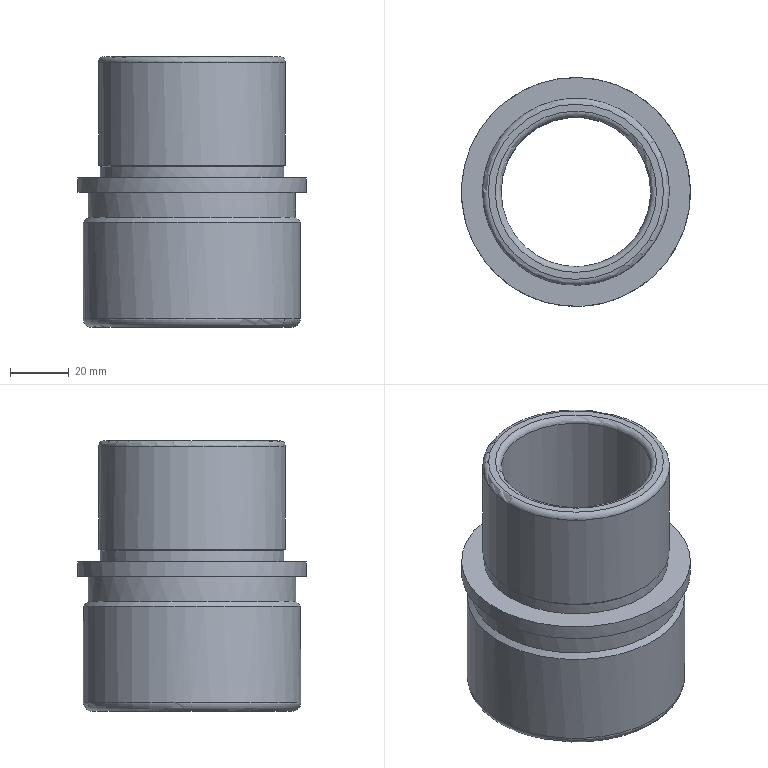Part | STEP file | 1_id1042_x_t | 1 solid | 16 faces | box 77.8 x 77.8 x 92.075 mm | volume 159468 mm3 | cylinder 6 | plane 4 | torus 4 | cone 2 | commonest cylinder face diameters 50.8 x1 62.484 x1 63.5 x1 70.62 x1 73.889 x1 77.8 x1
STEP:
#1=CARTESIAN_POINT('',(0.,0.,0.));
#2=DIRECTION('',(0.,0.,1.));
#3=DIRECTION('',(1.,0.,0.));
#4=AXIS2_PLACEMENT_3D('',#1,#2,#3);
#5=CARTESIAN_POINT('',(983.969,478.443,85.208));
#6=VERTEX_POINT('',#5);
#7=CARTESIAN_POINT('',(908.307,496.557,85.208));
#8=VERTEX_POINT('',#7);
#9=CARTESIAN_POINT('',(946.138,487.5,85.208));
#10=DIRECTION('',(0.,0.,-1.));
#11=DIRECTION('',(0.9725,-0.2328,0.));
#12=AXIS2_PLACEMENT_3D('',#9,#10,#11);
#13=CIRCLE('',#12,38.9);
#14=CARTESIAN_POINT('',(954.359,521.836,85.208));
#15=DIRECTION('',(0.,0.,1.));
#16=DIRECTION('',(0.,1.,0.));
#17=AXIS2_PLACEMENT_3D('',#14,#15,#16);
#18=PLANE('',#17);
#19=CARTESIAN_POINT('',(-43.393,-29.611));
#20=CARTESIAN_POINT('',(-108.918,-13.924));
#21=CARTESIAN_POINT('',(-62.57,34.979));
#22=CARTESIAN_POINT('',(-16.222,83.882));
#23=CARTESIAN_POINT('',(2.955,19.292));
#24=CARTESIAN_POINT('',(22.132,-45.298));
#25=CARTESIAN_POINT('',(-43.393,-29.611));
#26=(BOUNDED_CURVE()B_SPLINE_CURVE(2,(#19,#20,#21,#22,#23,#24,#25),.UNSPECIFIED.,.T.,.F.)B_SPLINE_CURVE_WITH_KNOTS((1,2,2,2,2,1),(-2.094,0.,2.094,4.189,6.283,8.378),.UNSPECIFIED.)CURVE()GEOMETRIC_REPRESENTATION_ITEM()RATIONAL_B_SPLINE_CURVE((1.,0.5,1.,0.5,1.,0.5,1.))REPRESENTATION_ITEM(''));
#27=(GEOMETRIC_REPRESENTATION_CONTEXT(2)PARAMETRIC_REPRESENTATION_CONTEXT()REPRESENTATION_CONTEXT('',''));
#28=DEFINITIONAL_REPRESENTATION('',(#26),#27);
#29=PCURVE('',#18,#28);
#30=CARTESIAN_POINT('',(946.138,487.5,125.11));
#31=DIRECTION('',(0.,0.,-1.));
#32=DIRECTION('',(-0.9725,0.2328,0.));
#33=AXIS2_PLACEMENT_3D('',#30,#31,#32);
#34=CYLINDRICAL_SURFACE('',#33,38.9);
#35=CARTESIAN_POINT('',(3.142,39.902));
#36=DIRECTION('',(1.,0.));
#37=VECTOR('',#36,1.);
#38=LINE('',#35,#37);
#39=(GEOMETRIC_REPRESENTATION_CONTEXT(2)PARAMETRIC_REPRESENTATION_CONTEXT()REPRESENTATION_CONTEXT('',''));
#40=DEFINITIONAL_REPRESENTATION('',(#38),#39);
#41=PCURVE('',#34,#40);
#42=SURFACE_CURVE('',#13,(#29,#41),.PCURVE_S1.);
#43=EDGE_CURVE('',#6,#8,#42,.T.);
#44=ORIENTED_EDGE('',*,*,#43,.T.);
#45=CARTESIAN_POINT('',(946.138,487.5,85.208));
#46=DIRECTION('',(0.,0.,-1.));
#47=DIRECTION('',(0.9725,-0.2328,0.));
#48=AXIS2_PLACEMENT_3D('',#45,#46,#47);
#49=CIRCLE('',#48,38.9);
#50=CARTESIAN_POINT('',(-43.393,-29.611));
#51=CARTESIAN_POINT('',(-108.918,-13.924));
#52=CARTESIAN_POINT('',(-62.57,34.979));
#53=CARTESIAN_POINT('',(-16.222,83.882));
#54=CARTESIAN_POINT('',(2.955,19.292));
#55=CARTESIAN_POINT('',(22.132,-45.298));
#56=CARTESIAN_POINT('',(-43.393,-29.611));
#57=(BOUNDED_CURVE()B_SPLINE_CURVE(2,(#50,#51,#52,#53,#54,#55,#56),.UNSPECIFIED.,.T.,.F.)B_SPLINE_CURVE_WITH_KNOTS((1,2,2,2,2,1),(-2.094,0.,2.094,4.189,6.283,8.378),.UNSPECIFIED.)CURVE()GEOMETRIC_REPRESENTATION_ITEM()RATIONAL_B_SPLINE_CURVE((1.,0.5,1.,0.5,1.,0.5,1.))REPRESENTATION_ITEM(''));
#58=(GEOMETRIC_REPRESENTATION_CONTEXT(2)PARAMETRIC_REPRESENTATION_CONTEXT()REPRESENTATION_CONTEXT('',''));
#59=DEFINITIONAL_REPRESENTATION('',(#57),#58);
#60=PCURVE('',#18,#59);
#61=CARTESIAN_POINT('',(-3.142,39.902));
#62=DIRECTION('',(1.,0.));
#63=VECTOR('',#62,1.);
#64=LINE('',#61,#63);
#65=(GEOMETRIC_REPRESENTATION_CONTEXT(2)PARAMETRIC_REPRESENTATION_CONTEXT()REPRESENTATION_CONTEXT('',''));
#66=DEFINITIONAL_REPRESENTATION('',(#64),#65);
#67=PCURVE('',#34,#66);
#68=SURFACE_CURVE('',#49,(#60,#67),.PCURVE_S1.);
#69=EDGE_CURVE('',#8,#6,#68,.T.);
#70=ORIENTED_EDGE('',*,*,#69,.T.);
#71=EDGE_LOOP('',(#44,#70));
#72=FACE_BOUND('',#71,.T.);
#73=CARTESIAN_POINT('',(980.478,479.279,85.208));
#74=VERTEX_POINT('',#73);
#75=CARTESIAN_POINT('',(946.138,487.5,85.208));
#76=DIRECTION('',(0.,0.,1.));
#77=DIRECTION('',(0.9725,-0.2328,0.));
#78=AXIS2_PLACEMENT_3D('',#75,#76,#77);
#79=CIRCLE('',#78,35.31);
#80=CARTESIAN_POINT('',(-34.336,8.22));
#81=DIRECTION('',(-0.2328,-0.9725));
#82=AXIS2_PLACEMENT_2D('',#80,#81);
#83=CIRCLE('',#82,35.31);
#84=(GEOMETRIC_REPRESENTATION_CONTEXT(2)PARAMETRIC_REPRESENTATION_CONTEXT()REPRESENTATION_CONTEXT('',''));
#85=DEFINITIONAL_REPRESENTATION('',(#83),#84);
#86=PCURVE('',#18,#85);
#87=CARTESIAN_POINT('',(946.138,487.5,76.762));
#88=DIRECTION('',(0.,0.,-1.));
#89=DIRECTION('',(0.9725,-0.2328,0.));
#90=AXIS2_PLACEMENT_3D('',#87,#88,#89);
#91=CYLINDRICAL_SURFACE('',#90,35.31);
#92=CARTESIAN_POINT('',(6.283,-8.446));
#93=DIRECTION('',(-1.,0.));
#94=VECTOR('',#93,1.);
#95=LINE('',#92,#94);
#96=(GEOMETRIC_REPRESENTATION_CONTEXT(2)PARAMETRIC_REPRESENTATION_CONTEXT()REPRESENTATION_CONTEXT('',''));
#97=DEFINITIONAL_REPRESENTATION('',(#95),#96);
#98=PCURVE('',#91,#97);
#99=SURFACE_CURVE('',#79,(#86,#98),.PCURVE_S1.);
#100=EDGE_CURVE('',#74,#74,#99,.T.);
#101=ORIENTED_EDGE('',*,*,#100,.T.);
#102=EDGE_LOOP('',(#101));
#103=FACE_BOUND('',#102,.T.);
#104=ADVANCED_FACE('',(#72,#103),#18,.F.);
#105=ORIENTED_EDGE('',*,*,#69,.F.);
#106=CARTESIAN_POINT('',(908.307,496.557,90.11));
#107=VERTEX_POINT('',#106);
#108=CARTESIAN_POINT('',(908.307,496.557,90.11));
#109=CARTESIAN_POINT('',(908.307,496.557,85.208));
#110=B_SPLINE_CURVE_WITH_KNOTS('',1,(#108,#109),.UNSPECIFIED.,.F.,.F.,(2,2),(35.,39.902),.PIECEWISE_BEZIER_KNOTS.);
#111=CARTESIAN_POINT('',(0.,0.));
#112=DIRECTION('',(0.,1.));
#113=VECTOR('',#112,1.);
#114=LINE('',#111,#113);
#115=(GEOMETRIC_REPRESENTATION_CONTEXT(2)PARAMETRIC_REPRESENTATION_CONTEXT()REPRESENTATION_CONTEXT('',''));
#116=DEFINITIONAL_REPRESENTATION('',(#114),#115);
#117=PCURVE('',#34,#116);
#118=CARTESIAN_POINT('',(6.283,0.));
#119=DIRECTION('',(0.,1.));
#120=VECTOR('',#119,1.);
#121=LINE('',#118,#120);
#122=(GEOMETRIC_REPRESENTATION_CONTEXT(2)PARAMETRIC_REPRESENTATION_CONTEXT()REPRESENTATION_CONTEXT('',''));
#123=DEFINITIONAL_REPRESENTATION('',(#121),#122);
#124=PCURVE('',#34,#123);
#125=SEAM_CURVE('',#110,(#117,#124),.PCURVE_S1.);
#126=EDGE_CURVE('',#107,#8,#125,.T.);
#127=ORIENTED_EDGE('',*,*,#126,.F.);
#128=CARTESIAN_POINT('',(946.138,487.5,90.11));
#129=DIRECTION('',(0.,0.,1.));
#130=DIRECTION('',(-0.9725,0.2328,0.));
#131=AXIS2_PLACEMENT_3D('',#128,#129,#130);
#132=CIRCLE('',#131,38.9);
#133=CARTESIAN_POINT('',(6.283,35.));
#134=DIRECTION('',(-1.,0.));
#135=VECTOR('',#134,1.);
#136=LINE('',#133,#135);
#137=(GEOMETRIC_REPRESENTATION_CONTEXT(2)PARAMETRIC_REPRESENTATION_CONTEXT()REPRESENTATION_CONTEXT('',''));
#138=DEFINITIONAL_REPRESENTATION('',(#136),#137);
#139=PCURVE('',#34,#138);
#140=CARTESIAN_POINT('',(954.869,523.969,90.11));
#141=DIRECTION('',(0.,0.,-1.));
#142=DIRECTION('',(0.,-1.,0.));
#143=AXIS2_PLACEMENT_3D('',#140,#141,#142);
#144=PLANE('',#143);
#145=CARTESIAN_POINT('',(27.413,46.562));
#146=CARTESIAN_POINT('',(92.938,62.249));
#147=CARTESIAN_POINT('',(73.76,-2.341));
#148=CARTESIAN_POINT('',(54.583,-66.931));
#149=CARTESIAN_POINT('',(8.235,-18.028));
#150=CARTESIAN_POINT('',(-38.113,30.875));
#151=CARTESIAN_POINT('',(27.413,46.562));
#152=(BOUNDED_CURVE()B_SPLINE_CURVE(2,(#145,#146,#147,#148,#149,#150,#151),.UNSPECIFIED.,.T.,.F.)B_SPLINE_CURVE_WITH_KNOTS((1,2,2,2,2,1),(-2.094,0.,2.094,4.189,6.283,8.378),.UNSPECIFIED.)CURVE()GEOMETRIC_REPRESENTATION_ITEM()RATIONAL_B_SPLINE_CURVE((1.,0.5,1.,0.5,1.,0.5,1.))REPRESENTATION_ITEM(''));
#153=(GEOMETRIC_REPRESENTATION_CONTEXT(2)PARAMETRIC_REPRESENTATION_CONTEXT()REPRESENTATION_CONTEXT('',''));
#154=DEFINITIONAL_REPRESENTATION('',(#152),#153);
#155=PCURVE('',#144,#154);
#156=SURFACE_CURVE('',#132,(#139,#155),.PCURVE_S1.);
#157=EDGE_CURVE('',#107,#107,#156,.T.);
#158=ORIENTED_EDGE('',*,*,#157,.F.);
#159=ORIENTED_EDGE('',*,*,#126,.T.);
#160=ORIENTED_EDGE('',*,*,#43,.F.);
#161=EDGE_LOOP('',(#105,#127,#158,#159,#160));
#162=FACE_BOUND('',#161,.T.);
#163=ADVANCED_FACE('',(#162),#34,.T.);
#164=ORIENTED_EDGE('',*,*,#157,.T.);
#165=EDGE_LOOP('',(#164));
#166=FACE_BOUND('',#165,.T.);
#167=CARTESIAN_POINT('',(976.522,480.226,90.11));
#168=VERTEX_POINT('',#167);
#169=CARTESIAN_POINT('',(915.755,494.774,90.11));
#170=VERTEX_POINT('',#169);
#171=CARTESIAN_POINT('',(946.138,487.5,90.11));
#172=DIRECTION('',(0.,0.,-1.));
#173=DIRECTION('',(0.9725,-0.2328,0.));
#174=AXIS2_PLACEMENT_3D('',#171,#172,#173);
#175=CIRCLE('',#174,31.242);
#176=CARTESIAN_POINT('',(36.469,8.731));
#177=DIRECTION('',(0.2328,-0.9725));
#178=AXIS2_PLACEMENT_2D('',#176,#177);
#179=CIRCLE('',#178,31.242);
#180=(GEOMETRIC_REPRESENTATION_CONTEXT(2)PARAMETRIC_REPRESENTATION_CONTEXT()REPRESENTATION_CONTEXT('',''));
#181=DEFINITIONAL_REPRESENTATION('',(#179),#180);
#182=PCURVE('',#144,#181);
#183=CARTESIAN_POINT('',(946.138,487.5,125.11));
#184=DIRECTION('',(0.,0.,-1.));
#185=DIRECTION('',(-0.9725,0.2328,0.));
#186=AXIS2_PLACEMENT_3D('',#183,#184,#185);
#187=CYLINDRICAL_SURFACE('',#186,31.242);
#188=CARTESIAN_POINT('',(3.142,35.));
#189=DIRECTION('',(1.,0.));
#190=VECTOR('',#189,1.);
#191=LINE('',#188,#190);
#192=(GEOMETRIC_REPRESENTATION_CONTEXT(2)PARAMETRIC_REPRESENTATION_CONTEXT()REPRESENTATION_CONTEXT('',''));
#193=DEFINITIONAL_REPRESENTATION('',(#191),#192);
#194=PCURVE('',#187,#193);
#195=SURFACE_CURVE('',#175,(#182,#194),.PCURVE_S1.);
#196=EDGE_CURVE('',#168,#170,#195,.T.);
#197=ORIENTED_EDGE('',*,*,#196,.T.);
#198=CARTESIAN_POINT('',(946.138,487.5,90.11));
#199=DIRECTION('',(0.,0.,-1.));
#200=DIRECTION('',(0.9725,-0.2328,0.));
#201=AXIS2_PLACEMENT_3D('',#198,#199,#200);
#202=CIRCLE('',#201,31.242);
#203=CARTESIAN_POINT('',(36.469,8.731));
#204=DIRECTION('',(0.2328,-0.9725));
#205=AXIS2_PLACEMENT_2D('',#203,#204);
#206=CIRCLE('',#205,31.242);
#207=(GEOMETRIC_REPRESENTATION_CONTEXT(2)PARAMETRIC_REPRESENTATION_CONTEXT()REPRESENTATION_CONTEXT('',''));
#208=DEFINITIONAL_REPRESENTATION('',(#206),#207);
#209=PCURVE('',#144,#208);
#210=CARTESIAN_POINT('',(-3.142,35.));
#211=DIRECTION('',(1.,0.));
#212=VECTOR('',#211,1.);
#213=LINE('',#210,#212);
#214=(GEOMETRIC_REPRESENTATION_CONTEXT(2)PARAMETRIC_REPRESENTATION_CONTEXT()REPRESENTATION_CONTEXT('',''));
#215=DEFINITIONAL_REPRESENTATION('',(#213),#214);
#216=PCURVE('',#187,#215);
#217=SURFACE_CURVE('',#202,(#209,#216),.PCURVE_S1.);
#218=EDGE_CURVE('',#170,#168,#217,.T.);
#219=ORIENTED_EDGE('',*,*,#218,.T.);
#220=EDGE_LOOP('',(#197,#219));
#221=FACE_BOUND('',#220,.T.);
#222=ADVANCED_FACE('',(#166,#221),#144,.F.);
#223=ORIENTED_EDGE('',*,*,#218,.F.);
#224=CARTESIAN_POINT('',(915.755,494.774,93.93));
#225=VERTEX_POINT('',#224);
#226=CARTESIAN_POINT('',(915.755,494.774,93.93));
#227=CARTESIAN_POINT('',(915.755,494.774,90.11));
#228=B_SPLINE_CURVE_WITH_KNOTS('',1,(#226,#227),.UNSPECIFIED.,.F.,.F.,(2,2),(31.18,35.),.PIECEWISE_BEZIER_KNOTS.);
#229=CARTESIAN_POINT('',(0.,0.));
#230=DIRECTION('',(0.,1.));
#231=VECTOR('',#230,1.);
#232=LINE('',#229,#231);
#233=(GEOMETRIC_REPRESENTATION_CONTEXT(2)PARAMETRIC_REPRESENTATION_CONTEXT()REPRESENTATION_CONTEXT('',''));
#234=DEFINITIONAL_REPRESENTATION('',(#232),#233);
#235=PCURVE('',#187,#234);
#236=CARTESIAN_POINT('',(6.283,0.));
#237=DIRECTION('',(0.,1.));
#238=VECTOR('',#237,1.);
#239=LINE('',#236,#238);
#240=(GEOMETRIC_REPRESENTATION_CONTEXT(2)PARAMETRIC_REPRESENTATION_CONTEXT()REPRESENTATION_CONTEXT('',''));
#241=DEFINITIONAL_REPRESENTATION('',(#239),#240);
#242=PCURVE('',#187,#241);
#243=SEAM_CURVE('',#228,(#235,#242),.PCURVE_S1.);
#244=EDGE_CURVE('',#225,#170,#243,.T.);
#245=ORIENTED_EDGE('',*,*,#244,.F.);
#246=CARTESIAN_POINT('',(946.138,487.5,93.93));
#247=DIRECTION('',(0.,0.,1.));
#248=DIRECTION('',(-0.9725,0.2328,0.));
#249=AXIS2_PLACEMENT_3D('',#246,#247,#248);
#250=CIRCLE('',#249,31.242);
#251=CARTESIAN_POINT('',(6.283,31.18));
#252=DIRECTION('',(-1.,0.));
#253=VECTOR('',#252,1.);
#254=LINE('',#251,#253);
#255=(GEOMETRIC_REPRESENTATION_CONTEXT(2)PARAMETRIC_REPRESENTATION_CONTEXT()REPRESENTATION_CONTEXT('',''));
#256=DEFINITIONAL_REPRESENTATION('',(#254),#255);
#257=PCURVE('',#187,#256);
#258=CARTESIAN_POINT('',(946.138,487.5,94.184));
#259=DIRECTION('',(0.,0.,1.));
#260=DIRECTION('',(-0.9725,0.2328,0.));
#261=AXIS2_PLACEMENT_3D('',#258,#259,#260);
#262=CONICAL_SURFACE('',#261,31.496,0.7854);
#263=CARTESIAN_POINT('',(0.,-0.254));
#264=DIRECTION('',(1.,0.));
#265=VECTOR('',#264,1.);
#266=LINE('',#263,#265);
#267=(GEOMETRIC_REPRESENTATION_CONTEXT(2)PARAMETRIC_REPRESENTATION_CONTEXT()REPRESENTATION_CONTEXT('',''));
#268=DEFINITIONAL_REPRESENTATION('',(#266),#267);
#269=PCURVE('',#262,#268);
#270=SURFACE_CURVE('',#250,(#257,#269),.PCURVE_S1.);
#271=EDGE_CURVE('',#225,#225,#270,.T.);
#272=ORIENTED_EDGE('',*,*,#271,.F.);
#273=ORIENTED_EDGE('',*,*,#244,.T.);
#274=ORIENTED_EDGE('',*,*,#196,.F.);
#275=EDGE_LOOP('',(#223,#245,#272,#273,#274));
#276=FACE_BOUND('',#275,.T.);
#277=ADVANCED_FACE('',(#276),#187,.T.);
#278=CARTESIAN_POINT('',(915.261,494.892,94.438));
#279=VERTEX_POINT('',#278);
#280=CARTESIAN_POINT('',(946.138,487.5,94.438));
#281=DIRECTION('',(0.,0.,-1.));
#282=DIRECTION('',(-0.9725,0.2328,0.));
#283=AXIS2_PLACEMENT_3D('',#280,#281,#282);
#284=CIRCLE('',#283,31.75);
#285=CARTESIAN_POINT('',(6.283,0.254));
#286=DIRECTION('',(-1.,0.));
#287=VECTOR('',#286,1.);
#288=LINE('',#285,#287);
#289=(GEOMETRIC_REPRESENTATION_CONTEXT(2)PARAMETRIC_REPRESENTATION_CONTEXT()REPRESENTATION_CONTEXT('',''));
#290=DEFINITIONAL_REPRESENTATION('',(#288),#289);
#291=PCURVE('',#262,#290);
#292=CARTESIAN_POINT('',(946.138,487.5,133.047));
#293=DIRECTION('',(0.,0.,-1.));
#294=DIRECTION('',(-0.9725,0.2328,0.));
#295=AXIS2_PLACEMENT_3D('',#292,#293,#294);
#296=CYLINDRICAL_SURFACE('',#295,31.75);
#297=CARTESIAN_POINT('',(0.,38.61));
#298=DIRECTION('',(1.,0.));
#299=VECTOR('',#298,1.);
#300=LINE('',#297,#299);
#301=(GEOMETRIC_REPRESENTATION_CONTEXT(2)PARAMETRIC_REPRESENTATION_CONTEXT()REPRESENTATION_CONTEXT('',''));
#302=DEFINITIONAL_REPRESENTATION('',(#300),#301);
#303=PCURVE('',#296,#302);
#304=SURFACE_CURVE('',#284,(#291,#303),.PCURVE_S1.);
#305=EDGE_CURVE('',#279,#279,#304,.T.);
#306=ORIENTED_EDGE('',*,*,#305,.T.);
#307=CARTESIAN_POINT('',(915.755,494.774,93.93));
#308=CARTESIAN_POINT('',(915.261,494.892,94.438));
#309=B_SPLINE_CURVE_WITH_KNOTS('',1,(#307,#308),.UNSPECIFIED.,.F.,.F.,(2,2),(-0.3592,0.3592),.PIECEWISE_BEZIER_KNOTS.);
#310=CARTESIAN_POINT('',(0.,0.));
#311=DIRECTION('',(0.,1.));
#312=VECTOR('',#311,1.);
#313=LINE('',#310,#312);
#314=(GEOMETRIC_REPRESENTATION_CONTEXT(2)PARAMETRIC_REPRESENTATION_CONTEXT()REPRESENTATION_CONTEXT('',''));
#315=DEFINITIONAL_REPRESENTATION('',(#313),#314);
#316=PCURVE('',#262,#315);
#317=CARTESIAN_POINT('',(6.283,0.));
#318=DIRECTION('',(0.,1.));
#319=VECTOR('',#318,1.);
#320=LINE('',#317,#319);
#321=(GEOMETRIC_REPRESENTATION_CONTEXT(2)PARAMETRIC_REPRESENTATION_CONTEXT()REPRESENTATION_CONTEXT('',''));
#322=DEFINITIONAL_REPRESENTATION('',(#320),#321);
#323=PCURVE('',#262,#322);
#324=SEAM_CURVE('',#309,(#316,#323),.PCURVE_S1.);
#325=EDGE_CURVE('',#225,#279,#324,.T.);
#326=ORIENTED_EDGE('',*,*,#325,.F.);
#327=ORIENTED_EDGE('',*,*,#271,.T.);
#328=ORIENTED_EDGE('',*,*,#325,.T.);
#329=EDGE_LOOP('',(#306,#326,#327,#328));
#330=FACE_BOUND('',#329,.T.);
#331=ADVANCED_FACE('',(#330),#262,.T.);
#332=ORIENTED_EDGE('',*,*,#305,.F.);
#333=CARTESIAN_POINT('',(915.261,494.892,129.385));
#334=VERTEX_POINT('',#333);
#335=CARTESIAN_POINT('',(915.261,494.892,129.385));
#336=CARTESIAN_POINT('',(915.261,494.892,94.438));
#337=B_SPLINE_CURVE_WITH_KNOTS('',1,(#335,#336),.UNSPECIFIED.,.F.,.F.,(2,2),(3.663,38.61),.PIECEWISE_BEZIER_KNOTS.);
#338=CARTESIAN_POINT('',(0.,0.));
#339=DIRECTION('',(0.,1.));
#340=VECTOR('',#339,1.);
#341=LINE('',#338,#340);
#342=(GEOMETRIC_REPRESENTATION_CONTEXT(2)PARAMETRIC_REPRESENTATION_CONTEXT()REPRESENTATION_CONTEXT('',''));
#343=DEFINITIONAL_REPRESENTATION('',(#341),#342);
#344=PCURVE('',#296,#343);
#345=CARTESIAN_POINT('',(6.283,0.));
#346=DIRECTION('',(0.,1.));
#347=VECTOR('',#346,1.);
#348=LINE('',#345,#347);
#349=(GEOMETRIC_REPRESENTATION_CONTEXT(2)PARAMETRIC_REPRESENTATION_CONTEXT()REPRESENTATION_CONTEXT('',''));
#350=DEFINITIONAL_REPRESENTATION('',(#348),#349);
#351=PCURVE('',#296,#350);
#352=SEAM_CURVE('',#337,(#344,#351),.PCURVE_S1.);
#353=EDGE_CURVE('',#334,#279,#352,.T.);
#354=ORIENTED_EDGE('',*,*,#353,.F.);
#355=CARTESIAN_POINT('',(977.888,487.5,129.385));
#356=VERTEX_POINT('',#355);
#357=CARTESIAN_POINT('',(946.138,487.5,129.385));
#358=DIRECTION('',(0.,0.,1.));
#359=DIRECTION('',(1.,0.,0.));
#360=AXIS2_PLACEMENT_3D('',#357,#358,#359);
#361=CIRCLE('',#360,31.75);
#362=CARTESIAN_POINT('',(2.907,3.663));
#363=DIRECTION('',(-1.,0.));
#364=VECTOR('',#363,1.);
#365=LINE('',#362,#364);
#366=(GEOMETRIC_REPRESENTATION_CONTEXT(2)PARAMETRIC_REPRESENTATION_CONTEXT()REPRESENTATION_CONTEXT('',''));
#367=DEFINITIONAL_REPRESENTATION('',(#365),#366);
#368=PCURVE('',#296,#367);
#369=CARTESIAN_POINT('',(946.138,487.5,129.385));
#370=DIRECTION('',(0.,0.,-1.));
#371=DIRECTION('',(1.,0.,0.));
#372=AXIS2_PLACEMENT_3D('',#369,#370,#371);
#373=TOROIDAL_SURFACE('',#372,29.75,2.);
#374=CARTESIAN_POINT('',(6.283,6.283));
#375=DIRECTION('',(-1.,0.));
#376=VECTOR('',#375,1.);
#377=LINE('',#374,#376);
#378=(GEOMETRIC_REPRESENTATION_CONTEXT(2)PARAMETRIC_REPRESENTATION_CONTEXT()REPRESENTATION_CONTEXT('',''));
#379=DEFINITIONAL_REPRESENTATION('',(#377),#378);
#380=PCURVE('',#373,#379);
#381=SURFACE_CURVE('',#361,(#368,#380),.PCURVE_S1.);
#382=EDGE_CURVE('',#356,#334,#381,.T.);
#383=ORIENTED_EDGE('',*,*,#382,.F.);
#384=CARTESIAN_POINT('',(946.138,487.5,129.385));
#385=DIRECTION('',(0.,0.,1.));
#386=DIRECTION('',(1.,0.,0.));
#387=AXIS2_PLACEMENT_3D('',#384,#385,#386);
#388=CIRCLE('',#387,31.75);
#389=CARTESIAN_POINT('',(9.19,3.663));
#390=DIRECTION('',(-1.,0.));
#391=VECTOR('',#390,1.);
#392=LINE('',#389,#391);
#393=(GEOMETRIC_REPRESENTATION_CONTEXT(2)PARAMETRIC_REPRESENTATION_CONTEXT()REPRESENTATION_CONTEXT('',''));
#394=DEFINITIONAL_REPRESENTATION('',(#392),#393);
#395=PCURVE('',#296,#394);
#396=CARTESIAN_POINT('',(6.283,6.283));
#397=DIRECTION('',(-1.,0.));
#398=VECTOR('',#397,1.);
#399=LINE('',#396,#398);
#400=(GEOMETRIC_REPRESENTATION_CONTEXT(2)PARAMETRIC_REPRESENTATION_CONTEXT()REPRESENTATION_CONTEXT('',''));
#401=DEFINITIONAL_REPRESENTATION('',(#399),#400);
#402=PCURVE('',#373,#401);
#403=SURFACE_CURVE('',#388,(#395,#402),.PCURVE_S1.);
#404=EDGE_CURVE('',#334,#356,#403,.T.);
#405=ORIENTED_EDGE('',*,*,#404,.F.);
#406=ORIENTED_EDGE('',*,*,#353,.T.);
#407=EDGE_LOOP('',(#332,#354,#383,#405,#406));
#408=FACE_BOUND('',#407,.T.);
#409=ADVANCED_FACE('',(#408),#296,.T.);
#410=ORIENTED_EDGE('',*,*,#382,.T.);
#411=ORIENTED_EDGE('',*,*,#404,.T.);
#412=CARTESIAN_POINT('',(975.888,487.5,131.385));
#413=VERTEX_POINT('',#412);
#414=CARTESIAN_POINT('',(975.888,487.5,131.385));
#415=CARTESIAN_POINT('',(976.423,487.5,131.385));
#416=CARTESIAN_POINT('',(976.944,487.5,131.215));
#417=CARTESIAN_POINT('',(977.392,487.5,130.889));
#418=CARTESIAN_POINT('',(977.718,487.5,130.44));
#419=CARTESIAN_POINT('',(977.888,487.5,129.92));
#420=CARTESIAN_POINT('',(977.888,487.5,129.385));
#421=(BOUNDED_CURVE()B_SPLINE_CURVE(6,(#414,#415,#416,#417,#418,#419,#420),.UNSPECIFIED.,.F.,.F.)B_SPLINE_CURVE_WITH_KNOTS((7,7),(-1.571,0.),.PIECEWISE_BEZIER_KNOTS.)CURVE()GEOMETRIC_REPRESENTATION_ITEM()RATIONAL_B_SPLINE_CURVE((1.031,1.01,0.9979,0.994,0.9979,1.01,1.031))REPRESENTATION_ITEM(''));
#422=CARTESIAN_POINT('',(0.,6.283));
#423=DIRECTION('',(0.,1.));
#424=VECTOR('',#423,1.);
#425=LINE('',#422,#424);
#426=(GEOMETRIC_REPRESENTATION_CONTEXT(2)PARAMETRIC_REPRESENTATION_CONTEXT()REPRESENTATION_CONTEXT('',''));
#427=DEFINITIONAL_REPRESENTATION('',(#425),#426);
#428=PCURVE('',#373,#427);
#429=CARTESIAN_POINT('',(6.283,6.283));
#430=DIRECTION('',(0.,1.));
#431=VECTOR('',#430,1.);
#432=LINE('',#429,#431);
#433=(GEOMETRIC_REPRESENTATION_CONTEXT(2)PARAMETRIC_REPRESENTATION_CONTEXT()REPRESENTATION_CONTEXT('',''));
#434=DEFINITIONAL_REPRESENTATION('',(#432),#433);
#435=PCURVE('',#373,#434);
#436=SEAM_CURVE('',#421,(#428,#435),.PCURVE_S1.);
#437=EDGE_CURVE('',#413,#356,#436,.T.);
#438=ORIENTED_EDGE('',*,*,#437,.F.);
#439=CARTESIAN_POINT('',(916.388,487.5,131.385));
#440=VERTEX_POINT('',#439);
#441=CARTESIAN_POINT('',(946.138,487.5,131.385));
#442=DIRECTION('',(0.,0.,1.));
#443=DIRECTION('',(-1.,0.,0.));
#444=AXIS2_PLACEMENT_3D('',#441,#442,#443);
#445=CIRCLE('',#444,29.75);
#446=CARTESIAN_POINT('',(3.142,4.712));
#447=DIRECTION('',(-1.,0.));
#448=VECTOR('',#447,1.);
#449=LINE('',#446,#448);
#450=(GEOMETRIC_REPRESENTATION_CONTEXT(2)PARAMETRIC_REPRESENTATION_CONTEXT()REPRESENTATION_CONTEXT('',''));
#451=DEFINITIONAL_REPRESENTATION('',(#449),#450);
#452=PCURVE('',#373,#451);
#453=CARTESIAN_POINT('',(953.24,-102.838,131.385));
#454=DIRECTION('',(0.,0.,-1.));
#455=DIRECTION('',(0.,-1.,0.));
#456=AXIS2_PLACEMENT_3D('',#453,#454,#455);
#457=PLANE('',#456);
#458=CARTESIAN_POINT('',(-590.338,36.851));
#459=CARTESIAN_POINT('',(-538.81,36.851));
#460=CARTESIAN_POINT('',(-564.574,-7.774));
#461=CARTESIAN_POINT('',(-590.338,-52.399));
#462=CARTESIAN_POINT('',(-616.102,-7.774));
#463=CARTESIAN_POINT('',(-641.867,36.851));
#464=CARTESIAN_POINT('',(-590.338,36.851));
#465=(BOUNDED_CURVE()B_SPLINE_CURVE(2,(#458,#459,#460,#461,#462,#463,#464),.UNSPECIFIED.,.T.,.F.)B_SPLINE_CURVE_WITH_KNOTS((1,2,2,2,2,1),(-2.094,0.,2.094,4.189,6.283,8.378),.UNSPECIFIED.)CURVE()GEOMETRIC_REPRESENTATION_ITEM()RATIONAL_B_SPLINE_CURVE((1.,0.5,1.,0.5,1.,0.5,1.))REPRESENTATION_ITEM(''));
#466=(GEOMETRIC_REPRESENTATION_CONTEXT(2)PARAMETRIC_REPRESENTATION_CONTEXT()REPRESENTATION_CONTEXT('',''));
#467=DEFINITIONAL_REPRESENTATION('',(#465),#466);
#468=PCURVE('',#457,#467);
#469=SURFACE_CURVE('',#445,(#452,#468),.PCURVE_S1.);
#470=EDGE_CURVE('',#440,#413,#469,.T.);
#471=ORIENTED_EDGE('',*,*,#470,.F.);
#472=CARTESIAN_POINT('',(946.138,487.5,131.385));
#473=DIRECTION('',(0.,0.,1.));
#474=DIRECTION('',(-1.,0.,0.));
#475=AXIS2_PLACEMENT_3D('',#472,#473,#474);
#476=CIRCLE('',#475,29.75);
#477=CARTESIAN_POINT('',(9.425,4.712));
#478=DIRECTION('',(-1.,0.));
#479=VECTOR('',#478,1.);
#480=LINE('',#477,#479);
#481=(GEOMETRIC_REPRESENTATION_CONTEXT(2)PARAMETRIC_REPRESENTATION_CONTEXT()REPRESENTATION_CONTEXT('',''));
#482=DEFINITIONAL_REPRESENTATION('',(#480),#481);
#483=PCURVE('',#373,#482);
#484=CARTESIAN_POINT('',(-590.338,36.851));
#485=CARTESIAN_POINT('',(-538.81,36.851));
#486=CARTESIAN_POINT('',(-564.574,-7.774));
#487=CARTESIAN_POINT('',(-590.338,-52.399));
#488=CARTESIAN_POINT('',(-616.102,-7.774));
#489=CARTESIAN_POINT('',(-641.867,36.851));
#490=CARTESIAN_POINT('',(-590.338,36.851));
#491=(BOUNDED_CURVE()B_SPLINE_CURVE(2,(#484,#485,#486,#487,#488,#489,#490),.UNSPECIFIED.,.T.,.F.)B_SPLINE_CURVE_WITH_KNOTS((1,2,2,2,2,1),(-2.094,0.,2.094,4.189,6.283,8.378),.UNSPECIFIED.)CURVE()GEOMETRIC_REPRESENTATION_ITEM()RATIONAL_B_SPLINE_CURVE((1.,0.5,1.,0.5,1.,0.5,1.))REPRESENTATION_ITEM(''));
#492=(GEOMETRIC_REPRESENTATION_CONTEXT(2)PARAMETRIC_REPRESENTATION_CONTEXT()REPRESENTATION_CONTEXT('',''));
#493=DEFINITIONAL_REPRESENTATION('',(#491),#492);
#494=PCURVE('',#457,#493);
#495=SURFACE_CURVE('',#476,(#483,#494),.PCURVE_S1.);
#496=EDGE_CURVE('',#413,#440,#495,.T.);
#497=ORIENTED_EDGE('',*,*,#496,.F.);
#498=ORIENTED_EDGE('',*,*,#437,.T.);
#499=EDGE_LOOP('',(#410,#411,#438,#471,#497,#498));
#500=FACE_BOUND('',#499,.T.);
#501=ADVANCED_FACE('',(#500),#373,.T.);
#502=ORIENTED_EDGE('',*,*,#470,.T.);
#503=ORIENTED_EDGE('',*,*,#496,.T.);
#504=EDGE_LOOP('',(#502,#503));
#505=FACE_BOUND('',#504,.T.);
#506=CARTESIAN_POINT('',(918.738,487.5,131.385));
#507=VERTEX_POINT('',#506);
#508=CARTESIAN_POINT('',(973.538,487.5,131.385));
#509=VERTEX_POINT('',#508);
#510=CARTESIAN_POINT('',(946.138,487.5,131.385));
#511=DIRECTION('',(0.,0.,-1.));
#512=DIRECTION('',(-1.,0.,0.));
#513=AXIS2_PLACEMENT_3D('',#510,#511,#512);
#514=CIRCLE('',#513,27.4);
#515=CARTESIAN_POINT('',(-590.338,7.101));
#516=DIRECTION('',(0.,1.));
#517=AXIS2_PLACEMENT_2D('',#515,#516);
#518=CIRCLE('',#517,27.4);
#519=(GEOMETRIC_REPRESENTATION_CONTEXT(2)PARAMETRIC_REPRESENTATION_CONTEXT()REPRESENTATION_CONTEXT('',''));
#520=DEFINITIONAL_REPRESENTATION('',(#518),#519);
#521=PCURVE('',#457,#520);
#522=CARTESIAN_POINT('',(946.138,487.5,129.385));
#523=DIRECTION('',(0.,0.,-1.));
#524=DIRECTION('',(1.,0.,0.));
#525=AXIS2_PLACEMENT_3D('',#522,#523,#524);
#526=TOROIDAL_SURFACE('',#525,27.4,2.);
#527=CARTESIAN_POINT('',(3.142,4.712));
#528=DIRECTION('',(1.,0.));
#529=VECTOR('',#528,1.);
#530=LINE('',#527,#529);
#531=(GEOMETRIC_REPRESENTATION_CONTEXT(2)PARAMETRIC_REPRESENTATION_CONTEXT()REPRESENTATION_CONTEXT('',''));
#532=DEFINITIONAL_REPRESENTATION('',(#530),#531);
#533=PCURVE('',#526,#532);
#534=SURFACE_CURVE('',#514,(#521,#533),.PCURVE_S1.);
#535=EDGE_CURVE('',#507,#509,#534,.T.);
#536=ORIENTED_EDGE('',*,*,#535,.T.);
#537=CARTESIAN_POINT('',(946.138,487.5,131.385));
#538=DIRECTION('',(0.,0.,-1.));
#539=DIRECTION('',(-1.,0.,0.));
#540=AXIS2_PLACEMENT_3D('',#537,#538,#539);
#541=CIRCLE('',#540,27.4);
#542=CARTESIAN_POINT('',(-590.338,7.101));
#543=DIRECTION('',(0.,1.));
#544=AXIS2_PLACEMENT_2D('',#542,#543);
#545=CIRCLE('',#544,27.4);
#546=(GEOMETRIC_REPRESENTATION_CONTEXT(2)PARAMETRIC_REPRESENTATION_CONTEXT()REPRESENTATION_CONTEXT('',''));
#547=DEFINITIONAL_REPRESENTATION('',(#545),#546);
#548=PCURVE('',#457,#547);
#549=CARTESIAN_POINT('',(-3.142,4.712));
#550=DIRECTION('',(1.,0.));
#551=VECTOR('',#550,1.);
#552=LINE('',#549,#551);
#553=(GEOMETRIC_REPRESENTATION_CONTEXT(2)PARAMETRIC_REPRESENTATION_CONTEXT()REPRESENTATION_CONTEXT('',''));
#554=DEFINITIONAL_REPRESENTATION('',(#552),#553);
#555=PCURVE('',#526,#554);
#556=SURFACE_CURVE('',#541,(#548,#555),.PCURVE_S1.);
#557=EDGE_CURVE('',#509,#507,#556,.T.);
#558=ORIENTED_EDGE('',*,*,#557,.T.);
#559=EDGE_LOOP('',(#536,#558));
#560=FACE_BOUND('',#559,.T.);
#561=ADVANCED_FACE('',(#505,#560),#457,.F.);
#562=ORIENTED_EDGE('',*,*,#557,.F.);
#563=CARTESIAN_POINT('',(971.538,487.5,129.385));
#564=VERTEX_POINT('',#563);
#565=CARTESIAN_POINT('',(971.538,487.5,129.385));
#566=CARTESIAN_POINT('',(971.538,487.5,129.92));
#567=CARTESIAN_POINT('',(971.708,487.5,130.44));
#568=CARTESIAN_POINT('',(972.035,487.5,130.889));
#569=CARTESIAN_POINT('',(972.483,487.5,131.215));
#570=CARTESIAN_POINT('',(973.004,487.5,131.385));
#571=CARTESIAN_POINT('',(973.538,487.5,131.385));
#572=(BOUNDED_CURVE()B_SPLINE_CURVE(6,(#565,#566,#567,#568,#569,#570,#571),.UNSPECIFIED.,.F.,.F.)B_SPLINE_CURVE_WITH_KNOTS((7,7),(3.142,4.712),.PIECEWISE_BEZIER_KNOTS.)CURVE()GEOMETRIC_REPRESENTATION_ITEM()RATIONAL_B_SPLINE_CURVE((1.031,1.01,0.9979,0.994,0.9979,1.01,1.031))REPRESENTATION_ITEM(''));
#573=CARTESIAN_POINT('',(0.,0.));
#574=DIRECTION('',(0.,1.));
#575=VECTOR('',#574,1.);
#576=LINE('',#573,#575);
#577=(GEOMETRIC_REPRESENTATION_CONTEXT(2)PARAMETRIC_REPRESENTATION_CONTEXT()REPRESENTATION_CONTEXT('',''));
#578=DEFINITIONAL_REPRESENTATION('',(#576),#577);
#579=PCURVE('',#526,#578);
#580=CARTESIAN_POINT('',(6.283,0.));
#581=DIRECTION('',(0.,1.));
#582=VECTOR('',#581,1.);
#583=LINE('',#580,#582);
#584=(GEOMETRIC_REPRESENTATION_CONTEXT(2)PARAMETRIC_REPRESENTATION_CONTEXT()REPRESENTATION_CONTEXT('',''));
#585=DEFINITIONAL_REPRESENTATION('',(#583),#584);
#586=PCURVE('',#526,#585);
#587=SEAM_CURVE('',#572,(#579,#586),.PCURVE_S1.);
#588=EDGE_CURVE('',#564,#509,#587,.T.);
#589=ORIENTED_EDGE('',*,*,#588,.F.);
#590=CARTESIAN_POINT('',(970.84,481.586,129.385));
#591=VERTEX_POINT('',#590);
#592=CARTESIAN_POINT('',(946.138,487.5,129.385));
#593=DIRECTION('',(0.,0.,-1.));
#594=DIRECTION('',(1.,0.,0.));
#595=AXIS2_PLACEMENT_3D('',#592,#593,#594);
#596=CIRCLE('',#595,25.4);
#597=CARTESIAN_POINT('',(0.,3.142));
#598=DIRECTION('',(1.,0.));
#599=VECTOR('',#598,1.);
#600=LINE('',#597,#599);
#601=(GEOMETRIC_REPRESENTATION_CONTEXT(2)PARAMETRIC_REPRESENTATION_CONTEXT()REPRESENTATION_CONTEXT('',''));
#602=DEFINITIONAL_REPRESENTATION('',(#600),#601);
#603=PCURVE('',#526,#602);
#604=CARTESIAN_POINT('',(946.138,487.5,158.047));
#605=DIRECTION('',(0.,0.,1.));
#606=DIRECTION('',(0.9725,-0.2328,0.));
#607=AXIS2_PLACEMENT_3D('',#604,#605,#606);
#608=CYLINDRICAL_SURFACE('',#607,25.4);
#609=CARTESIAN_POINT('',(0.235,-28.663));
#610=DIRECTION('',(-1.,0.));
#611=VECTOR('',#610,1.);
#612=LINE('',#609,#611);
#613=(GEOMETRIC_REPRESENTATION_CONTEXT(2)PARAMETRIC_REPRESENTATION_CONTEXT()REPRESENTATION_CONTEXT('',''));
#614=DEFINITIONAL_REPRESENTATION('',(#612),#613);
#615=PCURVE('',#608,#614);
#616=SURFACE_CURVE('',#596,(#603,#615),.PCURVE_S1.);
#617=EDGE_CURVE('',#564,#591,#616,.T.);
#618=ORIENTED_EDGE('',*,*,#617,.T.);
#619=CARTESIAN_POINT('',(946.138,487.5,129.385));
#620=DIRECTION('',(0.,0.,-1.));
#621=DIRECTION('',(1.,0.,0.));
#622=AXIS2_PLACEMENT_3D('',#619,#620,#621);
#623=CIRCLE('',#622,25.4);
#624=CARTESIAN_POINT('',(0.,3.142));
#625=DIRECTION('',(1.,0.));
#626=VECTOR('',#625,1.);
#627=LINE('',#624,#626);
#628=(GEOMETRIC_REPRESENTATION_CONTEXT(2)PARAMETRIC_REPRESENTATION_CONTEXT()REPRESENTATION_CONTEXT('',''));
#629=DEFINITIONAL_REPRESENTATION('',(#627),#628);
#630=PCURVE('',#526,#629);
#631=CARTESIAN_POINT('',(6.518,-28.663));
#632=DIRECTION('',(-1.,0.));
#633=VECTOR('',#632,1.);
#634=LINE('',#631,#633);
#635=(GEOMETRIC_REPRESENTATION_CONTEXT(2)PARAMETRIC_REPRESENTATION_CONTEXT()REPRESENTATION_CONTEXT('',''));
#636=DEFINITIONAL_REPRESENTATION('',(#634),#635);
#637=PCURVE('',#608,#636);
#638=SURFACE_CURVE('',#623,(#630,#637),.PCURVE_S1.);
#639=EDGE_CURVE('',#591,#564,#638,.T.);
#640=ORIENTED_EDGE('',*,*,#639,.T.);
#641=ORIENTED_EDGE('',*,*,#588,.T.);
#642=ORIENTED_EDGE('',*,*,#535,.F.);
#643=EDGE_LOOP('',(#562,#589,#618,#640,#641,#642));
#644=FACE_BOUND('',#643,.T.);
#645=ADVANCED_FACE('',(#644),#526,.T.);
#646=ORIENTED_EDGE('',*,*,#617,.T.);
#647=CARTESIAN_POINT('',(970.84,481.586,41.31));
#648=VERTEX_POINT('',#647);
#649=CARTESIAN_POINT('',(970.84,481.586,41.31));
#650=CARTESIAN_POINT('',(970.84,481.586,129.385));
#651=B_SPLINE_CURVE_WITH_KNOTS('',1,(#649,#650),.UNSPECIFIED.,.F.,.F.,(2,2),(-116.738,-28.663),.PIECEWISE_BEZIER_KNOTS.);
#652=CARTESIAN_POINT('',(0.,0.));
#653=DIRECTION('',(0.,1.));
#654=VECTOR('',#653,1.);
#655=LINE('',#652,#654);
#656=(GEOMETRIC_REPRESENTATION_CONTEXT(2)PARAMETRIC_REPRESENTATION_CONTEXT()REPRESENTATION_CONTEXT('',''));
#657=DEFINITIONAL_REPRESENTATION('',(#655),#656);
#658=PCURVE('',#608,#657);
#659=CARTESIAN_POINT('',(6.283,0.));
#660=DIRECTION('',(0.,1.));
#661=VECTOR('',#660,1.);
#662=LINE('',#659,#661);
#663=(GEOMETRIC_REPRESENTATION_CONTEXT(2)PARAMETRIC_REPRESENTATION_CONTEXT()REPRESENTATION_CONTEXT('',''));
#664=DEFINITIONAL_REPRESENTATION('',(#662),#663);
#665=PCURVE('',#608,#664);
#666=SEAM_CURVE('',#651,(#658,#665),.PCURVE_S1.);
#667=EDGE_CURVE('',#648,#591,#666,.T.);
#668=ORIENTED_EDGE('',*,*,#667,.F.);
#669=CARTESIAN_POINT('',(920.738,487.5,41.31));
#670=VERTEX_POINT('',#669);
#671=CARTESIAN_POINT('',(946.138,487.5,41.31));
#672=DIRECTION('',(0.,0.,1.));
#673=DIRECTION('',(0.9725,-0.2328,0.));
#674=AXIS2_PLACEMENT_3D('',#671,#672,#673);
#675=CIRCLE('',#674,25.4);
#676=CARTESIAN_POINT('',(0.,-116.738));
#677=DIRECTION('',(1.,0.));
#678=VECTOR('',#677,1.);
#679=LINE('',#676,#678);
#680=(GEOMETRIC_REPRESENTATION_CONTEXT(2)PARAMETRIC_REPRESENTATION_CONTEXT()REPRESENTATION_CONTEXT('',''));
#681=DEFINITIONAL_REPRESENTATION('',(#679),#680);
#682=PCURVE('',#608,#681);
#683=CARTESIAN_POINT('',(946.138,487.5,41.31));
#684=DIRECTION('',(0.,0.,1.));
#685=DIRECTION('',(-1.,0.,0.));
#686=AXIS2_PLACEMENT_3D('',#683,#684,#685);
#687=TOROIDAL_SURFACE('',#686,27.4,2.);
#688=CARTESIAN_POINT('',(2.907,3.142));
#689=DIRECTION('',(1.,0.));
#690=VECTOR('',#689,1.);
#691=LINE('',#688,#690);
#692=(GEOMETRIC_REPRESENTATION_CONTEXT(2)PARAMETRIC_REPRESENTATION_CONTEXT()REPRESENTATION_CONTEXT('',''));
#693=DEFINITIONAL_REPRESENTATION('',(#691),#692);
#694=PCURVE('',#687,#693);
#695=SURFACE_CURVE('',#675,(#682,#694),.PCURVE_S1.);
#696=EDGE_CURVE('',#648,#670,#695,.T.);
#697=ORIENTED_EDGE('',*,*,#696,.T.);
#698=CARTESIAN_POINT('',(946.138,487.5,41.31));
#699=DIRECTION('',(0.,0.,1.));
#700=DIRECTION('',(0.9725,-0.2328,0.));
#701=AXIS2_PLACEMENT_3D('',#698,#699,#700);
#702=CIRCLE('',#701,25.4);
#703=CARTESIAN_POINT('',(0.,-116.738));
#704=DIRECTION('',(1.,0.));
#705=VECTOR('',#704,1.);
#706=LINE('',#703,#705);
#707=(GEOMETRIC_REPRESENTATION_CONTEXT(2)PARAMETRIC_REPRESENTATION_CONTEXT()REPRESENTATION_CONTEXT('',''));
#708=DEFINITIONAL_REPRESENTATION('',(#706),#707);
#709=PCURVE('',#608,#708);
#710=CARTESIAN_POINT('',(-3.377,3.142));
#711=DIRECTION('',(1.,0.));
#712=VECTOR('',#711,1.);
#713=LINE('',#710,#712);
#714=(GEOMETRIC_REPRESENTATION_CONTEXT(2)PARAMETRIC_REPRESENTATION_CONTEXT()REPRESENTATION_CONTEXT('',''));
#715=DEFINITIONAL_REPRESENTATION('',(#713),#714);
#716=PCURVE('',#687,#715);
#717=SURFACE_CURVE('',#702,(#709,#716),.PCURVE_S1.);
#718=EDGE_CURVE('',#670,#648,#717,.T.);
#719=ORIENTED_EDGE('',*,*,#718,.T.);
#720=ORIENTED_EDGE('',*,*,#667,.T.);
#721=ORIENTED_EDGE('',*,*,#639,.T.);
#722=EDGE_LOOP('',(#646,#668,#697,#719,#720,#721));
#723=FACE_BOUND('',#722,.F.);
#724=ADVANCED_FACE('',(#723),#608,.F.);
#725=CARTESIAN_POINT('',(918.738,487.5,39.31));
#726=VERTEX_POINT('',#725);
#727=CARTESIAN_POINT('',(946.138,487.5,39.31));
#728=DIRECTION('',(0.,0.,1.));
#729=DIRECTION('',(-1.,0.,0.));
#730=AXIS2_PLACEMENT_3D('',#727,#728,#729);
#731=CIRCLE('',#730,27.4);
#732=CARTESIAN_POINT('',(0.,4.712));
#733=DIRECTION('',(1.,0.));
#734=VECTOR('',#733,1.);
#735=LINE('',#732,#734);
#736=(GEOMETRIC_REPRESENTATION_CONTEXT(2)PARAMETRIC_REPRESENTATION_CONTEXT()REPRESENTATION_CONTEXT('',''));
#737=DEFINITIONAL_REPRESENTATION('',(#735),#736);
#738=PCURVE('',#687,#737);
#739=CARTESIAN_POINT('',(946.138,-132.5,39.31));
#740=DIRECTION('',(0.,0.,1.));
#741=DIRECTION('',(0.,1.,0.));
#742=AXIS2_PLACEMENT_3D('',#739,#740,#741);
#743=PLANE('',#742);
#744=CARTESIAN_POINT('',(620.,0.));
#745=DIRECTION('',(0.,1.));
#746=AXIS2_PLACEMENT_2D('',#744,#745);
#747=CIRCLE('',#746,27.4);
#748=(GEOMETRIC_REPRESENTATION_CONTEXT(2)PARAMETRIC_REPRESENTATION_CONTEXT()REPRESENTATION_CONTEXT('',''));
#749=DEFINITIONAL_REPRESENTATION('',(#747),#748);
#750=PCURVE('',#743,#749);
#751=SURFACE_CURVE('',#731,(#738,#750),.PCURVE_S1.);
#752=EDGE_CURVE('',#726,#726,#751,.T.);
#753=ORIENTED_EDGE('',*,*,#752,.F.);
#754=CARTESIAN_POINT('',(920.738,487.5,41.31));
#755=CARTESIAN_POINT('',(920.738,487.5,40.775));
#756=CARTESIAN_POINT('',(920.568,487.5,40.255));
#757=CARTESIAN_POINT('',(920.242,487.5,39.806));
#758=CARTESIAN_POINT('',(919.794,487.5,39.48));
#759=CARTESIAN_POINT('',(919.273,487.5,39.31));
#760=CARTESIAN_POINT('',(918.738,487.5,39.31));
#761=(BOUNDED_CURVE()B_SPLINE_CURVE(6,(#754,#755,#756,#757,#758,#759,#760),.UNSPECIFIED.,.F.,.F.)B_SPLINE_CURVE_WITH_KNOTS((7,7),(3.142,4.712),.PIECEWISE_BEZIER_KNOTS.)CURVE()GEOMETRIC_REPRESENTATION_ITEM()RATIONAL_B_SPLINE_CURVE((1.031,1.01,0.9979,0.994,0.9979,1.01,1.031))REPRESENTATION_ITEM(''));
#762=CARTESIAN_POINT('',(0.,0.));
#763=DIRECTION('',(0.,1.));
#764=VECTOR('',#763,1.);
#765=LINE('',#762,#764);
#766=(GEOMETRIC_REPRESENTATION_CONTEXT(2)PARAMETRIC_REPRESENTATION_CONTEXT()REPRESENTATION_CONTEXT('',''));
#767=DEFINITIONAL_REPRESENTATION('',(#765),#766);
#768=PCURVE('',#687,#767);
#769=CARTESIAN_POINT('',(6.283,0.));
#770=DIRECTION('',(0.,1.));
#771=VECTOR('',#770,1.);
#772=LINE('',#769,#771);
#773=(GEOMETRIC_REPRESENTATION_CONTEXT(2)PARAMETRIC_REPRESENTATION_CONTEXT()REPRESENTATION_CONTEXT('',''));
#774=DEFINITIONAL_REPRESENTATION('',(#772),#773);
#775=PCURVE('',#687,#774);
#776=SEAM_CURVE('',#761,(#768,#775),.PCURVE_S1.);
#777=EDGE_CURVE('',#670,#726,#776,.T.);
#778=ORIENTED_EDGE('',*,*,#777,.F.);
#779=ORIENTED_EDGE('',*,*,#718,.T.);
#780=ORIENTED_EDGE('',*,*,#696,.T.);
#781=ORIENTED_EDGE('',*,*,#777,.T.);
#782=EDGE_LOOP('',(#753,#778,#779,#780,#781));
#783=FACE_BOUND('',#782,.T.);
#784=ADVANCED_FACE('',(#783),#687,.T.);
#785=CARTESIAN_POINT('',(980.083,487.5,39.31));
#786=VERTEX_POINT('',#785);
#787=CARTESIAN_POINT('',(912.194,487.5,39.31));
#788=VERTEX_POINT('',#787);
#789=CARTESIAN_POINT('',(946.138,487.5,39.31));
#790=DIRECTION('',(0.,0.,-1.));
#791=DIRECTION('',(1.,0.,0.));
#792=AXIS2_PLACEMENT_3D('',#789,#790,#791);
#793=CIRCLE('',#792,33.944);
#794=CARTESIAN_POINT('',(620.,-33.944));
#795=CARTESIAN_POINT('',(561.207,-33.944));
#796=CARTESIAN_POINT('',(590.603,16.972));
#797=CARTESIAN_POINT('',(620.,67.889));
#798=CARTESIAN_POINT('',(649.397,16.972));
#799=CARTESIAN_POINT('',(678.793,-33.944));
#800=CARTESIAN_POINT('',(620.,-33.944));
#801=(BOUNDED_CURVE()B_SPLINE_CURVE(2,(#794,#795,#796,#797,#798,#799,#800),.UNSPECIFIED.,.T.,.F.)B_SPLINE_CURVE_WITH_KNOTS((1,2,2,2,2,1),(-2.094,0.,2.094,4.189,6.283,8.378),.UNSPECIFIED.)CURVE()GEOMETRIC_REPRESENTATION_ITEM()RATIONAL_B_SPLINE_CURVE((1.,0.5,1.,0.5,1.,0.5,1.))REPRESENTATION_ITEM(''));
#802=(GEOMETRIC_REPRESENTATION_CONTEXT(2)PARAMETRIC_REPRESENTATION_CONTEXT()REPRESENTATION_CONTEXT('',''));
#803=DEFINITIONAL_REPRESENTATION('',(#801),#802);
#804=PCURVE('',#743,#803);
#805=CARTESIAN_POINT('',(946.138,487.5,42.31));
#806=DIRECTION('',(0.,0.,1.));
#807=DIRECTION('',(-1.,0.,0.));
#808=AXIS2_PLACEMENT_3D('',#805,#806,#807);
#809=TOROIDAL_SURFACE('',#808,33.944,3.);
#810=CARTESIAN_POINT('',(3.142,4.712));
#811=DIRECTION('',(-1.,0.));
#812=VECTOR('',#811,1.);
#813=LINE('',#810,#812);
#814=(GEOMETRIC_REPRESENTATION_CONTEXT(2)PARAMETRIC_REPRESENTATION_CONTEXT()REPRESENTATION_CONTEXT('',''));
#815=DEFINITIONAL_REPRESENTATION('',(#813),#814);
#816=PCURVE('',#809,#815);
#817=SURFACE_CURVE('',#793,(#804,#816),.PCURVE_S1.);
#818=EDGE_CURVE('',#786,#788,#817,.T.);
#819=ORIENTED_EDGE('',*,*,#818,.T.);
#820=CARTESIAN_POINT('',(946.138,487.5,39.31));
#821=DIRECTION('',(0.,0.,-1.));
#822=DIRECTION('',(1.,0.,0.));
#823=AXIS2_PLACEMENT_3D('',#820,#821,#822);
#824=CIRCLE('',#823,33.944);
#825=CARTESIAN_POINT('',(620.,-33.944));
#826=CARTESIAN_POINT('',(561.207,-33.944));
#827=CARTESIAN_POINT('',(590.603,16.972));
#828=CARTESIAN_POINT('',(620.,67.889));
#829=CARTESIAN_POINT('',(649.397,16.972));
#830=CARTESIAN_POINT('',(678.793,-33.944));
#831=CARTESIAN_POINT('',(620.,-33.944));
#832=(BOUNDED_CURVE()B_SPLINE_CURVE(2,(#825,#826,#827,#828,#829,#830,#831),.UNSPECIFIED.,.T.,.F.)B_SPLINE_CURVE_WITH_KNOTS((1,2,2,2,2,1),(-2.094,0.,2.094,4.189,6.283,8.378),.UNSPECIFIED.)CURVE()GEOMETRIC_REPRESENTATION_ITEM()RATIONAL_B_SPLINE_CURVE((1.,0.5,1.,0.5,1.,0.5,1.))REPRESENTATION_ITEM(''));
#833=(GEOMETRIC_REPRESENTATION_CONTEXT(2)PARAMETRIC_REPRESENTATION_CONTEXT()REPRESENTATION_CONTEXT('',''));
#834=DEFINITIONAL_REPRESENTATION('',(#832),#833);
#835=PCURVE('',#743,#834);
#836=CARTESIAN_POINT('',(9.425,4.712));
#837=DIRECTION('',(-1.,0.));
#838=VECTOR('',#837,1.);
#839=LINE('',#836,#838);
#840=(GEOMETRIC_REPRESENTATION_CONTEXT(2)PARAMETRIC_REPRESENTATION_CONTEXT()REPRESENTATION_CONTEXT('',''));
#841=DEFINITIONAL_REPRESENTATION('',(#839),#840);
#842=PCURVE('',#809,#841);
#843=SURFACE_CURVE('',#824,(#835,#842),.PCURVE_S1.);
#844=EDGE_CURVE('',#788,#786,#843,.T.);
#845=ORIENTED_EDGE('',*,*,#844,.T.);
#846=EDGE_LOOP('',(#819,#845));
#847=FACE_BOUND('',#846,.T.);
#848=ORIENTED_EDGE('',*,*,#752,.T.);
#849=EDGE_LOOP('',(#848));
#850=FACE_BOUND('',#849,.T.);
#851=ADVANCED_FACE('',(#847,#850),#743,.F.);
#852=CARTESIAN_POINT('',(909.194,487.5,42.31));
#853=VERTEX_POINT('',#852);
#854=CARTESIAN_POINT('',(910.209,496.101,42.31));
#855=VERTEX_POINT('',#854);
#856=CARTESIAN_POINT('',(946.138,487.5,42.31));
#857=DIRECTION('',(0.,0.,-1.));
#858=DIRECTION('',(-1.,0.,0.));
#859=AXIS2_PLACEMENT_3D('',#856,#857,#858);
#860=CIRCLE('',#859,36.944);
#861=CARTESIAN_POINT('',(6.283,6.283));
#862=DIRECTION('',(-1.,0.));
#863=VECTOR('',#862,1.);
#864=LINE('',#861,#863);
#865=(GEOMETRIC_REPRESENTATION_CONTEXT(2)PARAMETRIC_REPRESENTATION_CONTEXT()REPRESENTATION_CONTEXT('',''));
#866=DEFINITIONAL_REPRESENTATION('',(#864),#865);
#867=PCURVE('',#809,#866);
#868=CARTESIAN_POINT('',(946.138,487.5,125.11));
#869=DIRECTION('',(0.,0.,-1.));
#870=DIRECTION('',(-0.9725,0.2328,0.));
#871=AXIS2_PLACEMENT_3D('',#868,#869,#870);
#872=CYLINDRICAL_SURFACE('',#871,36.944);
#873=CARTESIAN_POINT('',(6.048,82.8));
#874=DIRECTION('',(1.,0.));
#875=VECTOR('',#874,1.);
#876=LINE('',#873,#875);
#877=(GEOMETRIC_REPRESENTATION_CONTEXT(2)PARAMETRIC_REPRESENTATION_CONTEXT()REPRESENTATION_CONTEXT('',''));
#878=DEFINITIONAL_REPRESENTATION('',(#876),#877);
#879=PCURVE('',#872,#878);
#880=SURFACE_CURVE('',#860,(#867,#879),.PCURVE_S1.);
#881=EDGE_CURVE('',#853,#855,#880,.T.);
#882=ORIENTED_EDGE('',*,*,#881,.T.);
#883=CARTESIAN_POINT('',(946.138,487.5,42.31));
#884=DIRECTION('',(0.,0.,-1.));
#885=DIRECTION('',(-1.,0.,0.));
#886=AXIS2_PLACEMENT_3D('',#883,#884,#885);
#887=CIRCLE('',#886,36.944);
#888=CARTESIAN_POINT('',(6.283,6.283));
#889=DIRECTION('',(-1.,0.));
#890=VECTOR('',#889,1.);
#891=LINE('',#888,#890);
#892=(GEOMETRIC_REPRESENTATION_CONTEXT(2)PARAMETRIC_REPRESENTATION_CONTEXT()REPRESENTATION_CONTEXT('',''));
#893=DEFINITIONAL_REPRESENTATION('',(#891),#892);
#894=PCURVE('',#809,#893);
#895=CARTESIAN_POINT('',(-0.235,82.8));
#896=DIRECTION('',(1.,0.));
#897=VECTOR('',#896,1.);
#898=LINE('',#895,#897);
#899=(GEOMETRIC_REPRESENTATION_CONTEXT(2)PARAMETRIC_REPRESENTATION_CONTEXT()REPRESENTATION_CONTEXT('',''));
#900=DEFINITIONAL_REPRESENTATION('',(#898),#899);
#901=PCURVE('',#872,#900);
#902=SURFACE_CURVE('',#887,(#894,#901),.PCURVE_S1.);
#903=EDGE_CURVE('',#855,#853,#902,.T.);
#904=ORIENTED_EDGE('',*,*,#903,.T.);
#905=CARTESIAN_POINT('',(912.194,487.5,39.31));
#906=CARTESIAN_POINT('',(911.392,487.5,39.31));
#907=CARTESIAN_POINT('',(910.611,487.5,39.565));
#908=CARTESIAN_POINT('',(909.938,487.5,40.054));
#909=CARTESIAN_POINT('',(909.449,487.5,40.727));
#910=CARTESIAN_POINT('',(909.194,487.5,41.508));
#911=CARTESIAN_POINT('',(909.194,487.5,42.31));
#912=(BOUNDED_CURVE()B_SPLINE_CURVE(6,(#905,#906,#907,#908,#909,#910,#911),.UNSPECIFIED.,.F.,.F.)B_SPLINE_CURVE_WITH_KNOTS((7,7),(-1.571,0.),.PIECEWISE_BEZIER_KNOTS.)CURVE()GEOMETRIC_REPRESENTATION_ITEM()RATIONAL_B_SPLINE_CURVE((1.031,1.01,0.9979,0.994,0.9979,1.01,1.031))REPRESENTATION_ITEM(''));
#913=CARTESIAN_POINT('',(0.,6.283));
#914=DIRECTION('',(0.,1.));
#915=VECTOR('',#914,1.);
#916=LINE('',#913,#915);
#917=(GEOMETRIC_REPRESENTATION_CONTEXT(2)PARAMETRIC_REPRESENTATION_CONTEXT()REPRESENTATION_CONTEXT('',''));
#918=DEFINITIONAL_REPRESENTATION('',(#916),#917);
#919=PCURVE('',#809,#918);
#920=CARTESIAN_POINT('',(6.283,6.283));
#921=DIRECTION('',(0.,1.));
#922=VECTOR('',#921,1.);
#923=LINE('',#920,#922);
#924=(GEOMETRIC_REPRESENTATION_CONTEXT(2)PARAMETRIC_REPRESENTATION_CONTEXT()REPRESENTATION_CONTEXT('',''));
#925=DEFINITIONAL_REPRESENTATION('',(#923),#924);
#926=PCURVE('',#809,#925);
#927=SEAM_CURVE('',#912,(#919,#926),.PCURVE_S1.);
#928=EDGE_CURVE('',#788,#853,#927,.T.);
#929=ORIENTED_EDGE('',*,*,#928,.F.);
#930=ORIENTED_EDGE('',*,*,#818,.F.);
#931=ORIENTED_EDGE('',*,*,#844,.F.);
#932=ORIENTED_EDGE('',*,*,#928,.T.);
#933=EDGE_LOOP('',(#882,#904,#929,#930,#931,#932));
#934=FACE_BOUND('',#933,.T.);
#935=ADVANCED_FACE('',(#934),#809,.T.);
#936=ORIENTED_EDGE('',*,*,#903,.F.);
#937=CARTESIAN_POINT('',(910.209,496.101,75.127));
#938=VERTEX_POINT('',#937);
#939=CARTESIAN_POINT('',(910.209,496.101,75.127));
#940=CARTESIAN_POINT('',(910.209,496.101,42.31));
#941=B_SPLINE_CURVE_WITH_KNOTS('',1,(#939,#940),.UNSPECIFIED.,.F.,.F.,(2,2),(49.983,82.8),.PIECEWISE_BEZIER_KNOTS.);
#942=CARTESIAN_POINT('',(0.,0.));
#943=DIRECTION('',(0.,1.));
#944=VECTOR('',#943,1.);
#945=LINE('',#942,#944);
#946=(GEOMETRIC_REPRESENTATION_CONTEXT(2)PARAMETRIC_REPRESENTATION_CONTEXT()REPRESENTATION_CONTEXT('',''));
#947=DEFINITIONAL_REPRESENTATION('',(#945),#946);
#948=PCURVE('',#872,#947);
#949=CARTESIAN_POINT('',(6.283,0.));
#950=DIRECTION('',(0.,1.));
#951=VECTOR('',#950,1.);
#952=LINE('',#949,#951);
#953=(GEOMETRIC_REPRESENTATION_CONTEXT(2)PARAMETRIC_REPRESENTATION_CONTEXT()REPRESENTATION_CONTEXT('',''));
#954=DEFINITIONAL_REPRESENTATION('',(#952),#953);
#955=PCURVE('',#872,#954);
#956=SEAM_CURVE('',#941,(#948,#955),.PCURVE_S1.);
#957=EDGE_CURVE('',#938,#855,#956,.T.);
#958=ORIENTED_EDGE('',*,*,#957,.F.);
#959=CARTESIAN_POINT('',(946.138,487.5,75.127));
#960=DIRECTION('',(0.,0.,1.));
#961=DIRECTION('',(-0.9725,0.2328,0.));
#962=AXIS2_PLACEMENT_3D('',#959,#960,#961);
#963=CIRCLE('',#962,36.944);
#964=CARTESIAN_POINT('',(6.283,49.983));
#965=DIRECTION('',(-1.,0.));
#966=VECTOR('',#965,1.);
#967=LINE('',#964,#966);
#968=(GEOMETRIC_REPRESENTATION_CONTEXT(2)PARAMETRIC_REPRESENTATION_CONTEXT()REPRESENTATION_CONTEXT('',''));
#969=DEFINITIONAL_REPRESENTATION('',(#967),#968);
#970=PCURVE('',#872,#969);
#971=CARTESIAN_POINT('',(946.138,487.5,75.945));
#972=DIRECTION('',(0.,0.,-1.));
#973=DIRECTION('',(0.9725,-0.2328,0.));
#974=AXIS2_PLACEMENT_3D('',#971,#972,#973);
#975=CONICAL_SURFACE('',#974,36.127,0.7854);
#976=CARTESIAN_POINT('',(9.425,0.8171));
#977=DIRECTION('',(-1.,0.));
#978=VECTOR('',#977,1.);
#979=LINE('',#976,#978);
#980=(GEOMETRIC_REPRESENTATION_CONTEXT(2)PARAMETRIC_REPRESENTATION_CONTEXT()REPRESENTATION_CONTEXT('',''));
#981=DEFINITIONAL_REPRESENTATION('',(#979),#980);
#982=PCURVE('',#975,#981);
#983=SURFACE_CURVE('',#963,(#970,#982),.PCURVE_S1.);
#984=EDGE_CURVE('',#938,#938,#983,.T.);
#985=ORIENTED_EDGE('',*,*,#984,.F.);
#986=ORIENTED_EDGE('',*,*,#957,.T.);
#987=ORIENTED_EDGE('',*,*,#881,.F.);
#988=EDGE_LOOP('',(#936,#958,#985,#986,#987));
#989=FACE_BOUND('',#988,.T.);
#990=ADVANCED_FACE('',(#989),#872,.T.);
#991=ORIENTED_EDGE('',*,*,#984,.T.);
#992=CARTESIAN_POINT('',(911.799,495.721,76.762));
#993=VERTEX_POINT('',#992);
#994=CARTESIAN_POINT('',(911.799,495.721,76.762));
#995=CARTESIAN_POINT('',(910.209,496.101,75.127));
#996=B_SPLINE_CURVE_WITH_KNOTS('',1,(#994,#995),.UNSPECIFIED.,.F.,.F.,(2,2),(-1.156,1.156),.PIECEWISE_BEZIER_KNOTS.);
#997=CARTESIAN_POINT('',(3.142,0.));
#998=DIRECTION('',(0.,1.));
#999=VECTOR('',#998,1.);
#1000=LINE('',#997,#999);
#1001=(GEOMETRIC_REPRESENTATION_CONTEXT(2)PARAMETRIC_REPRESENTATION_CONTEXT()REPRESENTATION_CONTEXT('',''));
#1002=DEFINITIONAL_REPRESENTATION('',(#1000),#1001);
#1003=PCURVE('',#975,#1002);
#1004=CARTESIAN_POINT('',(9.425,0.));
#1005=DIRECTION('',(0.,1.));
#1006=VECTOR('',#1005,1.);
#1007=LINE('',#1004,#1006);
#1008=(GEOMETRIC_REPRESENTATION_CONTEXT(2)PARAMETRIC_REPRESENTATION_CONTEXT()REPRESENTATION_CONTEXT('',''));
#1009=DEFINITIONAL_REPRESENTATION('',(#1007),#1008);
#1010=PCURVE('',#975,#1009);
#1011=SEAM_CURVE('',#996,(#1003,#1010),.PCURVE_S1.);
#1012=EDGE_CURVE('',#993,#938,#1011,.T.);
#1013=ORIENTED_EDGE('',*,*,#1012,.F.);
#1014=CARTESIAN_POINT('',(980.478,479.279,76.762));
#1015=VERTEX_POINT('',#1014);
#1016=CARTESIAN_POINT('',(946.138,487.5,76.762));
#1017=DIRECTION('',(0.,0.,-1.));
#1018=DIRECTION('',(-0.9725,0.2328,0.));
#1019=AXIS2_PLACEMENT_3D('',#1016,#1017,#1018);
#1020=CIRCLE('',#1019,35.31);
#1021=CARTESIAN_POINT('',(3.142,-0.8171));
#1022=DIRECTION('',(1.,0.));
#1023=VECTOR('',#1022,1.);
#1024=LINE('',#1021,#1023);
#1025=(GEOMETRIC_REPRESENTATION_CONTEXT(2)PARAMETRIC_REPRESENTATION_CONTEXT()REPRESENTATION_CONTEXT('',''));
#1026=DEFINITIONAL_REPRESENTATION('',(#1024),#1025);
#1027=PCURVE('',#975,#1026);
#1028=CARTESIAN_POINT('',(3.142,0.));
#1029=DIRECTION('',(1.,0.));
#1030=VECTOR('',#1029,1.);
#1031=LINE('',#1028,#1030);
#1032=(GEOMETRIC_REPRESENTATION_CONTEXT(2)PARAMETRIC_REPRESENTATION_CONTEXT()REPRESENTATION_CONTEXT('',''));
#1033=DEFINITIONAL_REPRESENTATION('',(#1031),#1032);
#1034=PCURVE('',#91,#1033);
#1035=SURFACE_CURVE('',#1020,(#1027,#1034),.PCURVE_S1.);
#1036=EDGE_CURVE('',#993,#1015,#1035,.T.);
#1037=ORIENTED_EDGE('',*,*,#1036,.T.);
#1038=CARTESIAN_POINT('',(946.138,487.5,76.762));
#1039=DIRECTION('',(0.,0.,-1.));
#1040=DIRECTION('',(-0.9725,0.2328,0.));
#1041=AXIS2_PLACEMENT_3D('',#1038,#1039,#1040);
#1042=CIRCLE('',#1041,35.31);
#1043=CARTESIAN_POINT('',(3.142,-0.8171));
#1044=DIRECTION('',(1.,0.));
#1045=VECTOR('',#1044,1.);
#1046=LINE('',#1043,#1045);
#1047=(GEOMETRIC_REPRESENTATION_CONTEXT(2)PARAMETRIC_REPRESENTATION_CONTEXT()REPRESENTATION_CONTEXT('',''));
#1048=DEFINITIONAL_REPRESENTATION('',(#1046),#1047);
#1049=PCURVE('',#975,#1048);
#1050=CARTESIAN_POINT('',(-3.142,0.));
#1051=DIRECTION('',(1.,0.));
#1052=VECTOR('',#1051,1.);
#1053=LINE('',#1050,#1052);
#1054=(GEOMETRIC_REPRESENTATION_CONTEXT(2)PARAMETRIC_REPRESENTATION_CONTEXT()REPRESENTATION_CONTEXT('',''));
#1055=DEFINITIONAL_REPRESENTATION('',(#1053),#1054);
#1056=PCURVE('',#91,#1055);
#1057=SURFACE_CURVE('',#1042,(#1049,#1056),.PCURVE_S1.);
#1058=EDGE_CURVE('',#1015,#993,#1057,.T.);
#1059=ORIENTED_EDGE('',*,*,#1058,.T.);
#1060=ORIENTED_EDGE('',*,*,#1012,.T.);
#1061=EDGE_LOOP('',(#991,#1013,#1037,#1059,#1060));
#1062=FACE_BOUND('',#1061,.T.);
#1063=ADVANCED_FACE('',(#1062),#975,.T.);
#1064=ORIENTED_EDGE('',*,*,#1058,.F.);
#1065=CARTESIAN_POINT('',(980.478,479.279,85.208));
#1066=CARTESIAN_POINT('',(980.478,479.279,76.762));
#1067=B_SPLINE_CURVE_WITH_KNOTS('',1,(#1065,#1066),.UNSPECIFIED.,.F.,.F.,(2,2),(-8.446,0.),.PIECEWISE_BEZIER_KNOTS.);
#1068=CARTESIAN_POINT('',(0.,0.));
#1069=DIRECTION('',(0.,1.));
#1070=VECTOR('',#1069,1.);
#1071=LINE('',#1068,#1070);
#1072=(GEOMETRIC_REPRESENTATION_CONTEXT(2)PARAMETRIC_REPRESENTATION_CONTEXT()REPRESENTATION_CONTEXT('',''));
#1073=DEFINITIONAL_REPRESENTATION('',(#1071),#1072);
#1074=PCURVE('',#91,#1073);
#1075=CARTESIAN_POINT('',(6.283,0.));
#1076=DIRECTION('',(0.,1.));
#1077=VECTOR('',#1076,1.);
#1078=LINE('',#1075,#1077);
#1079=(GEOMETRIC_REPRESENTATION_CONTEXT(2)PARAMETRIC_REPRESENTATION_CONTEXT()REPRESENTATION_CONTEXT('',''));
#1080=DEFINITIONAL_REPRESENTATION('',(#1078),#1079);
#1081=PCURVE('',#91,#1080);
#1082=SEAM_CURVE('',#1067,(#1074,#1081),.PCURVE_S1.);
#1083=EDGE_CURVE('',#74,#1015,#1082,.T.);
#1084=ORIENTED_EDGE('',*,*,#1083,.F.);
#1085=ORIENTED_EDGE('',*,*,#100,.F.);
#1086=ORIENTED_EDGE('',*,*,#1083,.T.);
#1087=ORIENTED_EDGE('',*,*,#1036,.F.);
#1088=EDGE_LOOP('',(#1064,#1084,#1085,#1086,#1087));
#1089=FACE_BOUND('',#1088,.T.);
#1090=ADVANCED_FACE('',(#1089),#91,.T.);
#1091=CLOSED_SHELL('',(#104,#163,#222,#277,#331,#409,#501,#561,#645,#724,#784,#851,#935,#990,#1063,#1090));
#1092=MANIFOLD_SOLID_BREP('',#1091);
#1093=(LENGTH_UNIT()NAMED_UNIT(*)SI_UNIT(.MILLI.,.METRE.));
#1094=UNCERTAINTY_MEASURE_WITH_UNIT(LENGTH_MEASURE(0.000005),#1093,'','');
#1095=(NAMED_UNIT(*)PLANE_ANGLE_UNIT()SI_UNIT($,.RADIAN.));
#1096=(NAMED_UNIT(*)SI_UNIT($,.STERADIAN.)SOLID_ANGLE_UNIT());
#1097=(GEOMETRIC_REPRESENTATION_CONTEXT(3)GLOBAL_UNCERTAINTY_ASSIGNED_CONTEXT((#1094))GLOBAL_UNIT_ASSIGNED_CONTEXT((#1093,#1095,#1096))REPRESENTATION_CONTEXT('',''));
#1098=ADVANCED_BREP_SHAPE_REPRESENTATION('',(#4,#1092),#1097);